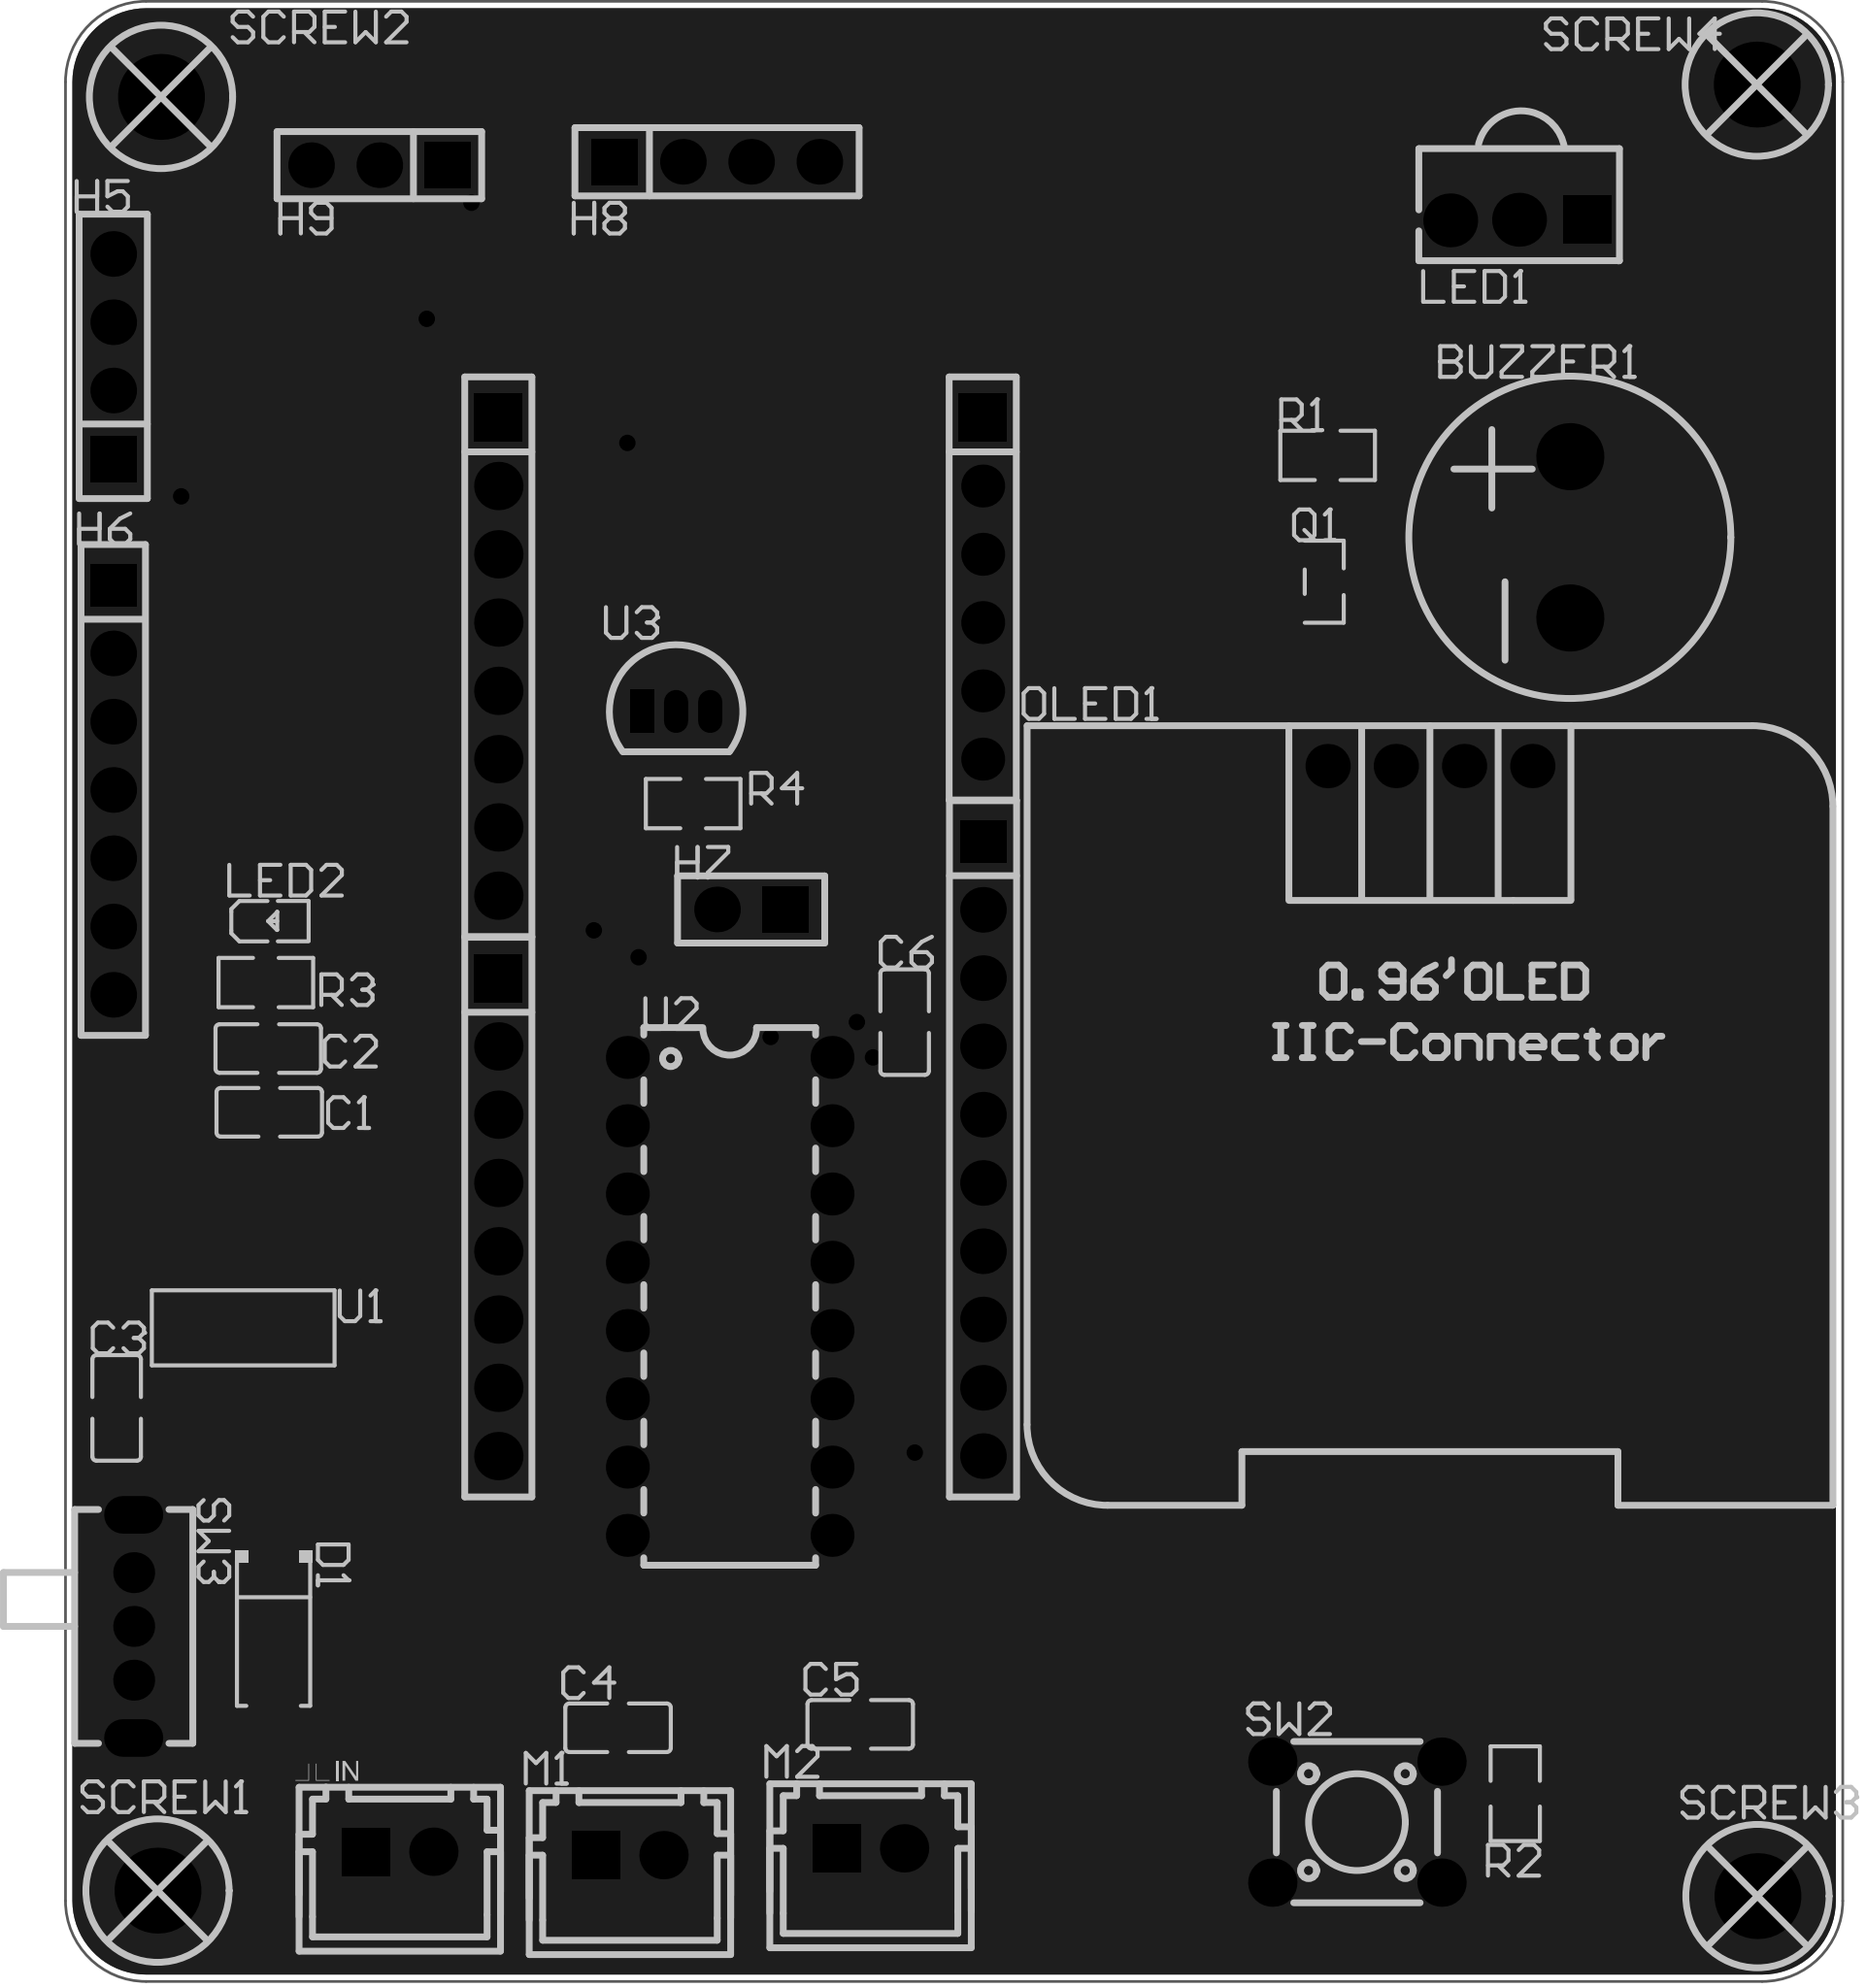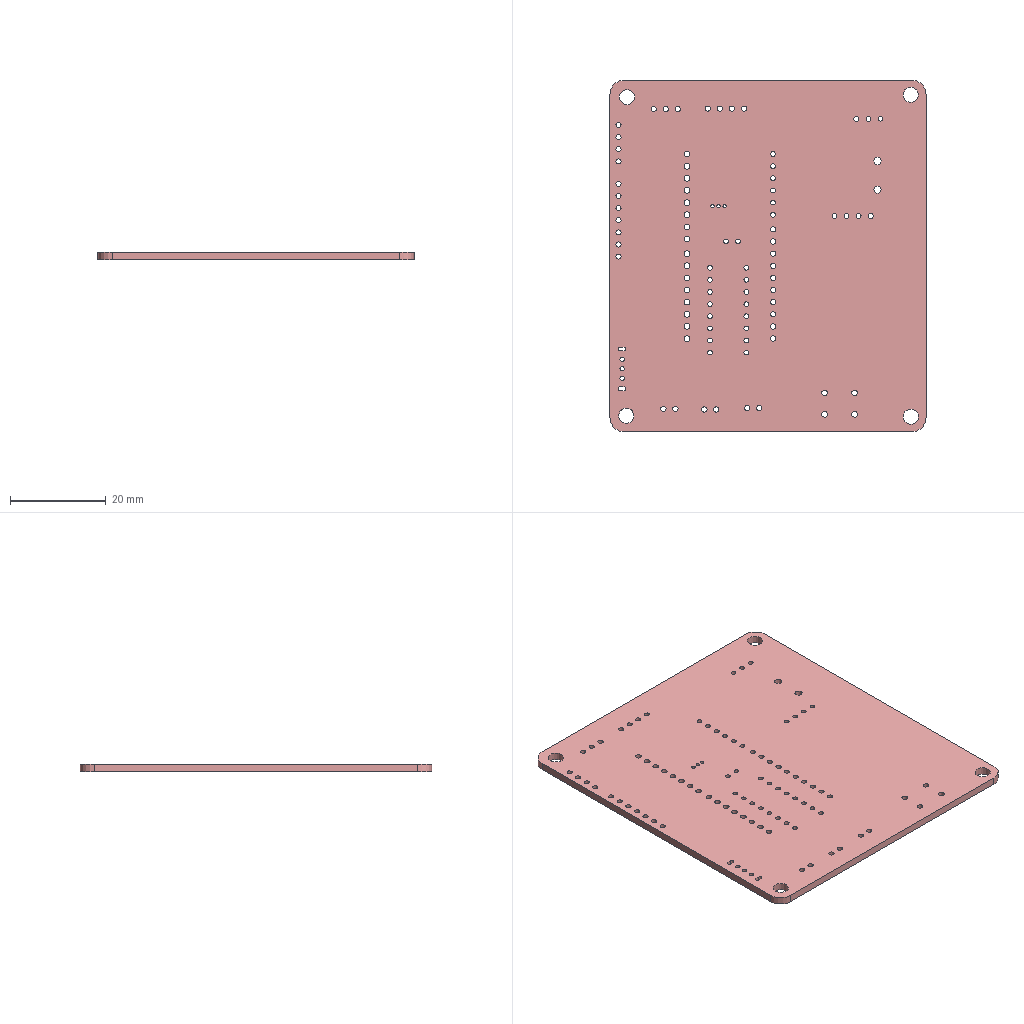Circuit board layout | Altium Designer | box 66.2 x 73.7 x 1.6 mm
Layer stack:
# Altium Designer layer stack of  (unit mm; dielectric type: 0 none, 1 core, 2 prepreg, 3 surface material)
index,name,kind,layer,copper_thickness_mm,dielectric_type,dielectric_thickness_mm,dielectric_material,dielectric_constant
0,Top Paste Mask Layer,other,,,,,,
1,Top Silkscreen Layer,other,,,,,,
2,Top Solder Mask Layer,dielectric,,,3,0.01,,3.3
3,Top Layer,copper,Top Layer,0.035,,,,
4,Dielectric1,dielectric,,,3,1.51,FR4,4.5
5,Bottom Layer,copper,Bottom Layer,0.035,,,,
6,Bottom Solder Mask Layer,dielectric,,,3,0.01,,3.3
7,Bottom Silkscreen Layer,other,,,,,,
8,Bottom Paste Mask Layer,other,,,,,,
# drill layer pairs: low layer,high layer
drill_pair,Top Layer,Bottom Layer
Part placement:
Designator,Comment,Layer,Footprint,Center-X(mm),Center-Y(mm),Rotation
BUZZER1,buzzer,TopLayer,BUZ-TH_BD12.0-P6.00-D0.9-RD,139.065,135.001,90
C1,10uF,TopLayer,C0805,90.644,113.613,180
C2,100nF,TopLayer,C0805,90.607,115.983,180
C3,10uF,TopLayer,C0805,84.963,102.616,270
C4,100nF,TopLayer,C0805,103.63,90.717,0
C5,100nF,TopLayer,C0805,112.646,90.844,0
C6,100nF,TopLayer,C0805,114.3,116.967,270
D1,SS14,TopLayer,SMA_L4.2-W2.6-LS5.3-RD,90.805,94.234,270
H1,,TopLayer,HDR-TH_8P-P2.54-V-F-1,99.172,130.56,270
H2,,TopLayer,HDR-TH_8P-P2.54-V-F-1,99.172,109.713,270
H3,,TopLayer,HDR-TH_6P-P2.54-V-F,117.207,133.1,270
H4,,TopLayer,HDR-TH_10P-P2.54-V-F,117.218,112.254,270
H5,,TopLayer,HDR-TH_4P-P2.54-V-F,84.836,141.732,90
H6,,TopLayer,HDR-TH_7P-P2.54-V-F,84.836,125.603,270
H7,,TopLayer,HDR-TH_2P-P2.54-V-F,108.585,121.158,180
H8,,TopLayer,HDR-TH_4P-P2.54-V-F,107.315,148.971,0
H9,,TopLayer,HDR-TH_3P-P2.54-V-M,94.742,148.844,180
LED1,TSDP34138,TopLayer,SENSOR-TH_TSDP34138,137.16,146.812,180
LED2,,TopLayer,LED_0603,90.72,120.717,0
M1,HX25003-2A,TopLayer,CONN-TH_2P-P2.50_HX25003-2A,104.072,85.979,0
M2,HX25003-2A,TopLayer,CONN-TH_2P-P2.50_HX25003-2A,113.03,86.233,0
OLED1,,TopLayer,0.96OLED_4P,133.858,126.492,0
Q1,SS8050,TopLayer,SOT-23-3_L2.9-W1.3-P1.90-LS2.4-BR,129.921,133.35,180
R1,200Ω,TopLayer,R0805,130.048,138.049,180
R2,4.7K,TopLayer,R0805,137.033,88.265,90
R3,4.7K,TopLayer,R0805,90.517,118.439,180
R4,4.7KΩ,TopLayer,R0805,106.426,125.095,0
SW2,TS1702-CZ65HBS,TopLayer,SW-TH_4P-L6.0-W6.0-P4.50-LS6.3,131.138,87.207,0
SW3,SK12D07VG4,TopLayer,SW-TH_SK12D07VG4,85.598,94.488,270
U1,AMS1117-5.0,TopLayer,SOT-223_L6.5-W3.5-P2.30-LS7.0-BR,89.674,105.594,90
U2,L293D,TopLayer,DIP-16_L20.0-W6.4-P2.54-LS7.6-BL,107.787,106.764,270
U3,DS18B20+,TopLayer,TO-92-3_L4.9-W3.7-P1.27-L,105.791,128.524,0
电源IN,HX25003-2A,TopLayer,CONN-TH_2P-P2.50_HX25003-2A,95.504,86.106,0
SCREW1,,TopLayer,M3螺丝,86.484,84.659,0
SCREW2,,TopLayer,M3螺丝,86.614,151.384,0
SCREW3,,TopLayer,M3螺丝,146.05,84.455,0
SCREW4,,TopLayer,M3螺丝,146.024,151.843,0
Pad and via stacks:
# Altium Designer via and pad stacks of  (unit mm). Each distinct definition once, with the count of objects using it.
# via: kind,start_layer,end_layer,hole_mm,diameter_mm,mode(0 simple;1 top-mid-bottom;2 full stack),diameter_per_layer,count,example_net
# pad: kind,layer,hole_mm,hole_type(0 round;1 square;2 slot),plating,top_size,top_shape(1 round;2 rect;3 octagon;9 rounded rect),mid_size,bottom_size,mode,footprint,size_per_layer,count,example
pad,Multi-Layer,1.5,0,plated,2.5x2.5,1,2.5x2.5,2.5x2.5,0,BUZ-TH_BD12.0-P6.00-D0.9-RD,,2,BUZZER1.1
pad,Multi-Layer,1.2,0,plated,1.8x1.8,2,1.8x1.8,1.8x1.8,0,HDR-TH_8P-P2.54-V-F-1,,2,H1.1
pad,Multi-Layer,1.2,0,plated,1.8x1.8,1,1.8x1.8,1.8x1.8,0,HDR-TH_8P-P2.54-V-F-1,,14,H1.2
pad,Multi-Layer,1.02,0,plated,1.6x1.6,1,1.6x1.6,1.6x1.6,0,HDR-TH_6P-P2.54-V-F,,5,H3.6
pad,Multi-Layer,1.02,0,plated,1.8x1.8,2,1.8x1.8,1.8x1.8,0,HDR-TH_6P-P2.54-V-F,,1,H3.1
pad,Multi-Layer,1.1,0,plated,1.7x1.7,1,1.7x1.7,1.7x1.7,0,HDR-TH_10P-P2.54-V-F,,9,H4.10
pad,Multi-Layer,1.1,0,plated,1.575x1.7,2,1.575x1.7,1.575x1.7,0,HDR-TH_10P-P2.54-V-F,,1,H4.1
pad,Multi-Layer,1.1,0,plated,1.7x1.7,2,1.7x1.7,1.7x1.7,0,HDR-TH_4P-P2.54-V-F,,2,H5.1
pad,Multi-Layer,1.1,0,plated,1.7x1.7,1,1.7x1.7,1.7x1.7,0,HDR-TH_4P-P2.54-V-F,,6,H5.2
pad,Multi-Layer,1.1,0,plated,1.7x1.7,1,1.7x1.7,1.7x1.7,0,HDR-TH_7P-P2.54-V-F,,6,H6.7
pad,Multi-Layer,1.1,0,plated,1.575x1.7,2,1.575x1.7,1.575x1.7,0,HDR-TH_7P-P2.54-V-F,,1,H6.1
pad,Multi-Layer,1,0,plated,1.7x1.7,2,1.7x1.7,1.7x1.7,0,HDR-TH_2P-P2.54-V-F,,1,H7.1
pad,Multi-Layer,1,0,plated,1.7x1.7,1,1.7x1.7,1.7x1.7,0,HDR-TH_2P-P2.54-V-F,,1,H7.2
pad,Multi-Layer,1.1,0,plated,1.7x1.7,2,1.7x1.7,1.7x1.7,0,HDR-TH_3P-P2.54-V-M,,1,H9.1
pad,Multi-Layer,1.1,0,plated,1.7x1.7,1,1.7x1.7,1.7x1.7,0,HDR-TH_3P-P2.54-V-M,,2,H9.2
pad,Multi-Layer,1.016,0,plated,2.007x2.007,1,2.007x2.007,2.007x2.007,0,SENSOR-TH_TSDP34138,,2,LED1.3
pad,Multi-Layer,1.016,0,plated,1.803x1.803,2,1.803x1.803,1.803x1.803,0,SENSOR-TH_TSDP34138,,1,LED1.1
pad,Multi-Layer,1.1,0,plated,1.8x1.8,2,1.8x1.8,1.8x1.8,0,CONN-TH_2P-P2.50_HX25003-2A,,3,M1.1
pad,Multi-Layer,1.1,0,plated,1.8x1.8,1,1.8x1.8,1.8x1.8,0,CONN-TH_2P-P2.50_HX25003-2A,,3,M1.2
pad,Multi-Layer,1,0,plated,1.65x1.65,1,1.65x1.65,1.65x1.65,0,0.96OLED_4P,,4,OLED1.4
pad,Multi-Layer,1.2,0,plated,1.8x1.8,1,1.8x1.8,1.8x1.8,0,SW-TH_4P-L6.0-W6.0-P4.50-LS6.3,,4,SW2.1
pad,Multi-Layer,0.9144,0,plated,1.524x1.524,1,1.524x1.524,1.524x1.524,0,SW-TH_SK12D07VG4,,3,SW3.1
pad,Multi-Layer,0.8,2,plated,1.4x2.2,1,1.4x2.2,1.4x2.2,0,SW-TH_SK12D07VG4,,2,SW3.4
pad,Multi-Layer,1,0,plated,1.6x1.6,1,1.6x1.6,1.6x1.6,0,DIP-16_L20.0-W6.4-P2.54-LS7.6-BL,,16,U2.1
pad,Multi-Layer,0.7,0,plated,0.9x1.6,1,0.9x1.6,0.9x1.6,0,TO-92-3_L4.9-W3.7-P1.27-L,,2,U3.3
pad,Multi-Layer,0.7,0,plated,0.9x1.6,2,0.9x1.6,0.9x1.6,0,TO-92-3_L4.9-W3.7-P1.27-L,,1,U3.1
pad,Multi-Layer,3.2,0,plated,3.2x3.2,1,3.2x3.2,3.2x3.2,0,M3\u00C2\u00DD\u00CB\u00BF,,4,SCREW1.1
pad,Top Layer,0,0,plated,1.41x1.35,2,1.41x1.35,1.41x1.35,0,C0805,,12,C1.2
pad,Top Layer,0,0,plated,2.2x1.7,2,2.2x1.7,2.2x1.7,0,SMA_L4.2-W2.6-LS5.3-RD,,2,D1.1
pad,Top Layer,0,0,plated,0.8001x0.8001,2,0.8001x0.8001,0.8001x0.8001,0,LED_0603,,2,LED2.1
pad,Top Layer,0,0,plated,1.25x0.7,2,1.25x0.7,1.25x0.7,0,SOT-23-3_L2.9-W1.3-P1.90-LS2.4-BR,,3,Q1.1
pad,Top Layer,0,0,plated,1.133x1.377,2,1.133x1.377,1.133x1.377,0,R0805,,8,R1.2
pad,Top Layer,0,0,plated,2.465x1.05,2,2.465x1.05,2.465x1.05,0,SOT-223_L6.5-W3.5-P2.30-LS7.0-BR,,3,U1.1
pad,Top Layer,0,0,plated,2.465x3.54,2,2.465x3.54,2.465x3.54,0,SOT-223_L6.5-W3.5-P2.30-LS7.0-BR,,1,U1.4
via,Top Layer,Bottom Layer,0.3048,0.61,0,,4,3.3V
via,Top Layer,Bottom Layer,0.3048,0.6096,0,,6,+5V
Copper pours:
name,layer,net,type(0 solid;1 hatched;2 none)
Top Layer-GND,Top Layer,GND,0
Bottom Layer-GND,Bottom Layer,GND,0
Design rules, without the lines most boards share:
# Altium Designer design rules of  (exported by Altium Designer, unit mm)
# columns: name | kind | enabled | priority | scope1 | scope2 | descriptor | typed fields (field=value)
copperThickness2oz | 0 | disabled | 1 | All | All | Clearance Constraint (Gap=6mil) (Disabled)(All),(All) | gap=0.1524
Plane_innerPlane | 0 | disabled | 2 | All | All | Clearance Constraint (Gap=6mil) (Disabled)(All),(All) | gap=0.1524
Copper_copperRegion | 0 | disabled | 3 | All | All | Clearance Constraint (Gap=6mil) (Disabled)(All),(All) | gap=0.1524
copperThickness1oz | 0 | enabled | 4 | All | All | Clearance Constraint (Gap=6mil) (All),(All) | gap=0.1524
otherClearance | 52 | enabled | 1 | All | All | Hole To Hole Clearance (Gap=11.8mil) (All),(All) | gap=0.2997
copperThickness1oz_2 | 2 | enabled | 2 | All | All | Width Constraint (Min=20mil) (Max=100mil) (Preferred=30mil) (All) |
viaSize | 11 | enabled | 1 | All | All | Routing Via (MinHoleWidth=11.8mil) (MaxHoleWidth=248mil) (PreferredHoleWidth=12mil) (MinWidth=19.7mil) (MaxWidth=393.7mil) (PreferedWidth=24mil) (All) | via_min_hole=0.2997 via_max_hole=6.299 via_preferred_diameter=0.6096 via_preferred_hole=0.3048